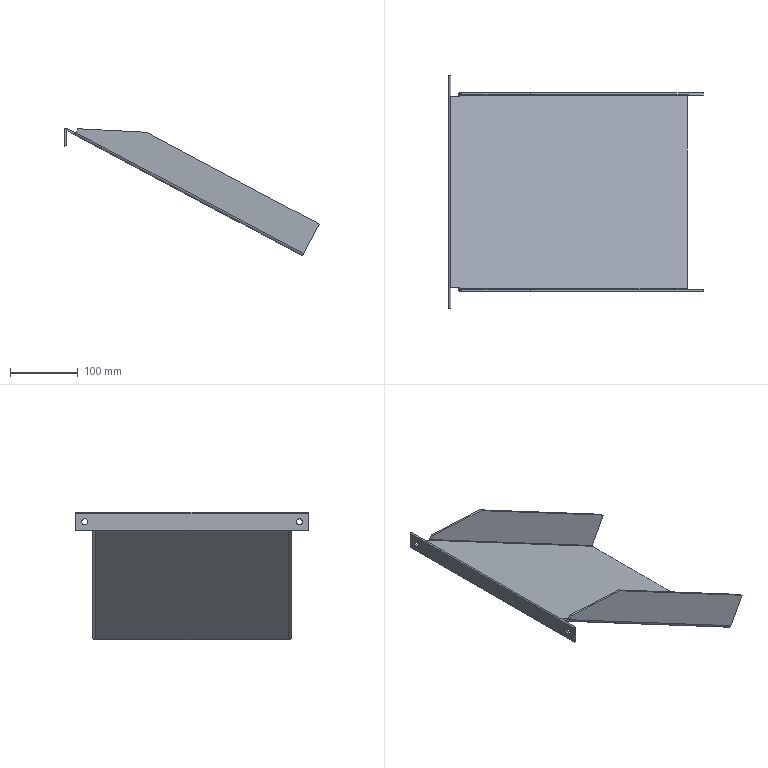Part | STEP file | lll_id3810_x_t | 1 solid | 27 faces | box 374.192 x 342 x 188.133 mm | volume 469805 mm3 | plane 20 | cylinder 7 | commonest cylinder face diameters 2 x2 8 x2 9 x2 3 x1
STEP:
#1=CARTESIAN_POINT('',(230.435,126.,-181.5));
#2=VERTEX_POINT('',#1);
#3=CARTESIAN_POINT('',(230.435,96.,-181.5));
#4=VERTEX_POINT('',#3);
#5=CARTESIAN_POINT('',(230.435,36.,-181.5));
#6=DIRECTION('',(0.,-1.,0.));
#7=VECTOR('',#6,1.);
#8=LINE('',#5,#7);
#9=EDGE_CURVE('',#2,#4,#8,.T.);
#10=ORIENTED_EDGE('',*,*,#9,.T.);
#11=CARTESIAN_POINT('',(230.435,96.,-183.996));
#12=VERTEX_POINT('',#11);
#13=CARTESIAN_POINT('',(230.435,96.,-193.833));
#14=DIRECTION('',(0.,0.,-1.));
#15=VECTOR('',#14,1.);
#16=LINE('',#13,#15);
#17=EDGE_CURVE('',#4,#12,#16,.T.);
#18=ORIENTED_EDGE('',*,*,#17,.T.);
#19=CARTESIAN_POINT('',(230.435,-186.,-183.996));
#20=VERTEX_POINT('',#19);
#21=CARTESIAN_POINT('',(230.435,-45.,-183.996));
#22=DIRECTION('',(0.,-1.,0.));
#23=VECTOR('',#22,1.);
#24=LINE('',#21,#23);
#25=EDGE_CURVE('',#12,#20,#24,.T.);
#26=ORIENTED_EDGE('',*,*,#25,.T.);
#27=CARTESIAN_POINT('',(230.435,-186.,-181.5));
#28=VERTEX_POINT('',#27);
#29=CARTESIAN_POINT('',(230.435,-186.,-193.833));
#30=DIRECTION('',(0.,0.,1.));
#31=VECTOR('',#30,1.);
#32=LINE('',#29,#31);
#33=EDGE_CURVE('',#20,#28,#32,.T.);
#34=ORIENTED_EDGE('',*,*,#33,.T.);
#35=CARTESIAN_POINT('',(230.435,-216.,-181.5));
#36=VERTEX_POINT('',#35);
#37=CARTESIAN_POINT('',(230.435,-201.,-181.5));
#38=DIRECTION('',(0.,-1.,0.));
#39=VECTOR('',#38,1.);
#40=LINE('',#37,#39);
#41=EDGE_CURVE('',#28,#36,#40,.T.);
#42=ORIENTED_EDGE('',*,*,#41,.T.);
#43=CARTESIAN_POINT('',(230.435,-216.,-206.128));
#44=VERTEX_POINT('',#43);
#45=CARTESIAN_POINT('',(230.435,-216.,-193.833));
#46=DIRECTION('',(0.,0.,1.));
#47=VECTOR('',#46,1.);
#48=LINE('',#45,#47);
#49=EDGE_CURVE('',#44,#36,#48,.T.);
#50=ORIENTED_EDGE('',*,*,#49,.F.);
#51=CARTESIAN_POINT('',(230.435,126.,-206.128));
#52=VERTEX_POINT('',#51);
#53=CARTESIAN_POINT('',(230.435,285.,-206.128));
#54=DIRECTION('',(0.,-1.,0.));
#55=VECTOR('',#54,1.);
#56=LINE('',#53,#55);
#57=EDGE_CURVE('',#52,#44,#56,.T.);
#58=ORIENTED_EDGE('',*,*,#57,.F.);
#59=CARTESIAN_POINT('',(230.435,126.,-193.833));
#60=DIRECTION('',(0.,0.,-1.));
#61=VECTOR('',#60,1.);
#62=LINE('',#59,#61);
#63=EDGE_CURVE('',#2,#52,#62,.T.);
#64=ORIENTED_EDGE('',*,*,#63,.F.);
#65=EDGE_LOOP('',(#10,#18,#26,#34,#42,#50,#58,#64));
#66=FACE_BOUND('',#65,.T.);
#67=CARTESIAN_POINT('',(230.435,113.,-189.565));
#68=VERTEX_POINT('',#67);
#69=CARTESIAN_POINT('',(230.435,113.,-194.083));
#70=DIRECTION('',(1.,0.,0.));
#71=DIRECTION('',(0.,0.,-1.));
#72=AXIS2_PLACEMENT_3D('',#69,#70,#71);
#73=ELLIPSE('',#72,4.517,4.5);
#74=EDGE_CURVE('',#68,#68,#73,.T.);
#75=ORIENTED_EDGE('',*,*,#74,.F.);
#76=EDGE_LOOP('',(#75));
#77=FACE_BOUND('',#76,.T.);
#78=CARTESIAN_POINT('',(230.435,-203.,-189.565));
#79=VERTEX_POINT('',#78);
#80=CARTESIAN_POINT('',(230.435,-203.,-194.083));
#81=DIRECTION('',(1.,0.,0.));
#82=DIRECTION('',(0.,0.,-1.));
#83=AXIS2_PLACEMENT_3D('',#80,#81,#82);
#84=ELLIPSE('',#83,4.517,4.5);
#85=EDGE_CURVE('',#79,#79,#84,.T.);
#86=ORIENTED_EDGE('',*,*,#85,.F.);
#87=EDGE_LOOP('',(#86));
#88=FACE_BOUND('',#87,.T.);
#89=CARTESIAN_POINT('',(230.435,-45.,-193.833));
#90=DIRECTION('',(1.,0.,0.));
#91=DIRECTION('',(0.,0.,-1.));
#92=AXIS2_PLACEMENT_3D('',#89,#90,#91);
#93=PLANE('',#92);
#94=ADVANCED_FACE('',(#66,#77,#88),#93,.T.);
#95=CARTESIAN_POINT('',(227.435,-216.,-206.391));
#96=VERTEX_POINT('',#95);
#97=CARTESIAN_POINT('',(227.435,-216.,-181.5));
#98=VERTEX_POINT('',#97);
#99=CARTESIAN_POINT('',(227.435,-216.,-173.216));
#100=DIRECTION('',(0.,0.,1.));
#101=VECTOR('',#100,1.);
#102=LINE('',#99,#101);
#103=EDGE_CURVE('',#96,#98,#102,.T.);
#104=ORIENTED_EDGE('',*,*,#103,.T.);
#105=CARTESIAN_POINT('',(227.435,126.,-181.5));
#106=VERTEX_POINT('',#105);
#107=CARTESIAN_POINT('',(227.435,-45.,-181.5));
#108=DIRECTION('',(0.,1.,0.));
#109=VECTOR('',#108,1.);
#110=LINE('',#107,#109);
#111=EDGE_CURVE('',#98,#106,#110,.T.);
#112=ORIENTED_EDGE('',*,*,#111,.T.);
#113=CARTESIAN_POINT('',(227.435,126.,-206.391));
#114=VERTEX_POINT('',#113);
#115=CARTESIAN_POINT('',(227.435,126.,-178.749));
#116=DIRECTION('',(0.,0.,-1.));
#117=VECTOR('',#116,1.);
#118=LINE('',#115,#117);
#119=EDGE_CURVE('',#106,#114,#118,.T.);
#120=ORIENTED_EDGE('',*,*,#119,.T.);
#121=CARTESIAN_POINT('',(227.435,110.,-206.391));
#122=DIRECTION('',(0.,-1.,0.));
#123=VECTOR('',#122,1.);
#124=LINE('',#121,#123);
#125=EDGE_CURVE('',#114,#96,#124,.T.);
#126=ORIENTED_EDGE('',*,*,#125,.T.);
#127=EDGE_LOOP('',(#104,#112,#120,#126));
#128=FACE_BOUND('',#127,.T.);
#129=CARTESIAN_POINT('',(227.435,113.,-198.862));
#130=VERTEX_POINT('',#129);
#131=CARTESIAN_POINT('',(227.435,113.,-194.345));
#132=DIRECTION('',(1.,0.,0.));
#133=DIRECTION('',(0.,0.,-1.));
#134=AXIS2_PLACEMENT_3D('',#131,#132,#133);
#135=ELLIPSE('',#134,4.517,4.5);
#136=EDGE_CURVE('',#130,#130,#135,.T.);
#137=ORIENTED_EDGE('',*,*,#136,.T.);
#138=EDGE_LOOP('',(#137));
#139=FACE_BOUND('',#138,.T.);
#140=CARTESIAN_POINT('',(227.435,-203.,-198.862));
#141=VERTEX_POINT('',#140);
#142=CARTESIAN_POINT('',(227.435,-203.,-194.345));
#143=DIRECTION('',(1.,0.,0.));
#144=DIRECTION('',(0.,0.,-1.));
#145=AXIS2_PLACEMENT_3D('',#142,#143,#144);
#146=ELLIPSE('',#145,4.517,4.5);
#147=EDGE_CURVE('',#141,#141,#146,.T.);
#148=ORIENTED_EDGE('',*,*,#147,.T.);
#149=EDGE_LOOP('',(#148));
#150=FACE_BOUND('',#149,.T.);
#151=CARTESIAN_POINT('',(227.435,110.,-170.446));
#152=DIRECTION('',(-1.,0.,0.));
#153=DIRECTION('',(0.,0.,-1.));
#154=AXIS2_PLACEMENT_3D('',#151,#152,#153);
#155=PLANE('',#154);
#156=ADVANCED_FACE('',(#128,#139,#150),#155,.T.);
#157=ORIENTED_EDGE('',*,*,#63,.T.);
#158=CARTESIAN_POINT('',(229.591,126.,-206.202));
#159=DIRECTION('',(-0.9962,0.,-0.08716));
#160=VECTOR('',#159,1.);
#161=LINE('',#158,#160);
#162=EDGE_CURVE('',#52,#114,#161,.T.);
#163=ORIENTED_EDGE('',*,*,#162,.T.);
#164=ORIENTED_EDGE('',*,*,#119,.F.);
#165=CARTESIAN_POINT('',(228.935,126.,-181.5));
#166=DIRECTION('',(0.,1.,0.));
#167=DIRECTION('',(-0.9962,0.,-0.08716));
#168=AXIS2_PLACEMENT_3D('',#165,#166,#167);
#169=CIRCLE('',#168,1.5);
#170=EDGE_CURVE('',#106,#2,#169,.T.);
#171=ORIENTED_EDGE('',*,*,#170,.T.);
#172=EDGE_LOOP('',(#157,#163,#164,#171));
#173=FACE_OUTER_BOUND('',#172,.T.);
#174=CARTESIAN_POINT('',(246.792,126.,-178.749));
#175=DIRECTION('',(0.,-1.,0.));
#176=DIRECTION('',(0.4226,0.,0.9063));
#177=AXIS2_PLACEMENT_3D('',#174,#175,#176);
#178=PLANE('',#177);
#179=ADVANCED_FACE('',(#173),#178,.F.);
#180=CARTESIAN_POINT('',(229.591,-216.,-206.202));
#181=DIRECTION('',(-0.9962,0.,-0.08716));
#182=VECTOR('',#181,1.);
#183=LINE('',#180,#182);
#184=EDGE_CURVE('',#44,#96,#183,.T.);
#185=ORIENTED_EDGE('',*,*,#184,.T.);
#186=ORIENTED_EDGE('',*,*,#125,.F.);
#187=ORIENTED_EDGE('',*,*,#162,.F.);
#188=ORIENTED_EDGE('',*,*,#57,.T.);
#189=EDGE_LOOP('',(#185,#186,#187,#188));
#190=FACE_OUTER_BOUND('',#189,.T.);
#191=CARTESIAN_POINT('',(229.591,285.,-206.202));
#192=DIRECTION('',(0.08716,0.,-0.9962));
#193=DIRECTION('',(0.,-1.,0.));
#194=AXIS2_PLACEMENT_3D('',#191,#192,#193);
#195=PLANE('',#194);
#196=ADVANCED_FACE('',(#190),#195,.T.);
#197=ORIENTED_EDGE('',*,*,#103,.F.);
#198=ORIENTED_EDGE('',*,*,#184,.F.);
#199=ORIENTED_EDGE('',*,*,#49,.T.);
#200=CARTESIAN_POINT('',(228.935,-216.,-181.5));
#201=DIRECTION('',(0.,-1.,0.));
#202=DIRECTION('',(-0.08716,0.,0.9962));
#203=AXIS2_PLACEMENT_3D('',#200,#201,#202);
#204=CIRCLE('',#203,1.5);
#205=EDGE_CURVE('',#36,#98,#204,.T.);
#206=ORIENTED_EDGE('',*,*,#205,.T.);
#207=EDGE_LOOP('',(#197,#198,#199,#206));
#208=FACE_OUTER_BOUND('',#207,.T.);
#209=CARTESIAN_POINT('',(226.705,-216.,-173.216));
#210=DIRECTION('',(0.,1.,0.));
#211=DIRECTION('',(0.08716,0.,-0.9962));
#212=AXIS2_PLACEMENT_3D('',#209,#210,#211);
#213=PLANE('',#212);
#214=ADVANCED_FACE('',(#208),#213,.F.);
#215=CARTESIAN_POINT('',(229.639,-186.,-180.176));
#216=VERTEX_POINT('',#215);
#217=CARTESIAN_POINT('',(242.945,-186.,-187.25));
#218=VERTEX_POINT('',#217);
#219=CARTESIAN_POINT('',(223.069,-186.,-176.682));
#220=DIRECTION('',(0.8829,0.,-0.4695));
#221=VECTOR('',#220,1.);
#222=LINE('',#219,#221);
#223=EDGE_CURVE('',#216,#218,#222,.T.);
#224=ORIENTED_EDGE('',*,*,#223,.T.);
#225=CARTESIAN_POINT('',(242.945,-187.,-187.25));
#226=VERTEX_POINT('',#225);
#227=CARTESIAN_POINT('',(242.945,92.,-187.25));
#228=DIRECTION('',(0.,-1.,0.));
#229=VECTOR('',#228,1.);
#230=LINE('',#227,#229);
#231=EDGE_CURVE('',#218,#226,#230,.T.);
#232=ORIENTED_EDGE('',*,*,#231,.T.);
#233=CARTESIAN_POINT('',(578.154,-187.,-365.484));
#234=VERTEX_POINT('',#233);
#235=CARTESIAN_POINT('',(228.807,-187.,-179.733));
#236=DIRECTION('',(0.8829,0.,-0.4695));
#237=VECTOR('',#236,1.);
#238=LINE('',#235,#237);
#239=EDGE_CURVE('',#226,#234,#238,.T.);
#240=ORIENTED_EDGE('',*,*,#239,.T.);
#241=CARTESIAN_POINT('',(578.154,97.,-365.484));
#242=VERTEX_POINT('',#241);
#243=CARTESIAN_POINT('',(578.154,-35.,-365.484));
#244=DIRECTION('',(0.,1.,0.));
#245=VECTOR('',#244,1.);
#246=LINE('',#243,#245);
#247=EDGE_CURVE('',#234,#242,#246,.T.);
#248=ORIENTED_EDGE('',*,*,#247,.T.);
#249=CARTESIAN_POINT('',(242.945,97.,-187.25));
#250=VERTEX_POINT('',#249);
#251=CARTESIAN_POINT('',(228.807,97.,-179.733));
#252=DIRECTION('',(-0.8829,0.,0.4695));
#253=VECTOR('',#252,1.);
#254=LINE('',#251,#253);
#255=EDGE_CURVE('',#242,#250,#254,.T.);
#256=ORIENTED_EDGE('',*,*,#255,.T.);
#257=CARTESIAN_POINT('',(242.945,96.,-187.25));
#258=VERTEX_POINT('',#257);
#259=CARTESIAN_POINT('',(242.945,-289.,-187.25));
#260=DIRECTION('',(0.,-1.,0.));
#261=VECTOR('',#260,1.);
#262=LINE('',#259,#261);
#263=EDGE_CURVE('',#250,#258,#262,.T.);
#264=ORIENTED_EDGE('',*,*,#263,.T.);
#265=CARTESIAN_POINT('',(229.639,96.,-180.176));
#266=VERTEX_POINT('',#265);
#267=CARTESIAN_POINT('',(228.631,96.,-179.64));
#268=DIRECTION('',(-0.8829,0.,0.4695));
#269=VECTOR('',#268,1.);
#270=LINE('',#267,#269);
#271=EDGE_CURVE('',#258,#266,#270,.T.);
#272=ORIENTED_EDGE('',*,*,#271,.T.);
#273=CARTESIAN_POINT('',(229.639,-45.,-180.176));
#274=DIRECTION('',(0.,-1.,0.));
#275=VECTOR('',#274,1.);
#276=LINE('',#273,#275);
#277=EDGE_CURVE('',#266,#216,#276,.T.);
#278=ORIENTED_EDGE('',*,*,#277,.T.);
#279=EDGE_LOOP('',(#224,#232,#240,#248,#256,#264,#272,#278));
#280=FACE_OUTER_BOUND('',#279,.T.);
#281=CARTESIAN_POINT('',(228.807,-35.,-179.733));
#282=DIRECTION('',(0.4695,0.,0.8829));
#283=DIRECTION('',(0.8829,0.,-0.4695));
#284=AXIS2_PLACEMENT_3D('',#281,#282,#283);
#285=PLANE('',#284);
#286=ADVANCED_FACE('',(#280),#285,.T.);
#287=ORIENTED_EDGE('',*,*,#271,.F.);
#288=CARTESIAN_POINT('',(241.537,96.,-189.899));
#289=VERTEX_POINT('',#288);
#290=CARTESIAN_POINT('',(242.945,96.,-187.25));
#291=DIRECTION('',(0.4695,0.,0.8829));
#292=VECTOR('',#291,1.);
#293=LINE('',#290,#292);
#294=EDGE_CURVE('',#289,#258,#293,.T.);
#295=ORIENTED_EDGE('',*,*,#294,.F.);
#296=CARTESIAN_POINT('',(227.399,96.,-182.382));
#297=DIRECTION('',(-0.8829,0.,0.4695));
#298=VECTOR('',#297,1.);
#299=LINE('',#296,#298);
#300=EDGE_CURVE('',#289,#12,#299,.T.);
#301=ORIENTED_EDGE('',*,*,#300,.T.);
#302=ORIENTED_EDGE('',*,*,#17,.F.);
#303=CARTESIAN_POINT('',(228.935,96.,-181.5));
#304=DIRECTION('',(0.,-1.,0.));
#305=DIRECTION('',(0.08716,0.,-0.9962));
#306=AXIS2_PLACEMENT_3D('',#303,#304,#305);
#307=CIRCLE('',#306,1.5);
#308=EDGE_CURVE('',#4,#266,#307,.T.);
#309=ORIENTED_EDGE('',*,*,#308,.T.);
#310=EDGE_LOOP('',(#287,#295,#301,#302,#309));
#311=FACE_OUTER_BOUND('',#310,.T.);
#312=CARTESIAN_POINT('',(228.563,96.,-179.768));
#313=DIRECTION('',(0.,-1.,0.));
#314=DIRECTION('',(0.9397,0.,-0.342));
#315=AXIS2_PLACEMENT_3D('',#312,#313,#314);
#316=PLANE('',#315);
#317=ADVANCED_FACE('',(#311),#316,.F.);
#318=CARTESIAN_POINT('',(228.935,-186.,-181.5));
#319=DIRECTION('',(0.,1.,0.));
#320=DIRECTION('',(0.9962,0.,0.08716));
#321=AXIS2_PLACEMENT_3D('',#318,#319,#320);
#322=CIRCLE('',#321,1.5);
#323=EDGE_CURVE('',#216,#28,#322,.T.);
#324=ORIENTED_EDGE('',*,*,#323,.T.);
#325=ORIENTED_EDGE('',*,*,#33,.F.);
#326=CARTESIAN_POINT('',(241.537,-186.,-189.899));
#327=VERTEX_POINT('',#326);
#328=CARTESIAN_POINT('',(227.399,-186.,-182.382));
#329=DIRECTION('',(0.8829,0.,-0.4695));
#330=VECTOR('',#329,1.);
#331=LINE('',#328,#330);
#332=EDGE_CURVE('',#20,#327,#331,.T.);
#333=ORIENTED_EDGE('',*,*,#332,.T.);
#334=CARTESIAN_POINT('',(242.945,-186.,-187.25));
#335=DIRECTION('',(0.4695,0.,0.8829));
#336=VECTOR('',#335,1.);
#337=LINE('',#334,#336);
#338=EDGE_CURVE('',#327,#218,#337,.T.);
#339=ORIENTED_EDGE('',*,*,#338,.T.);
#340=ORIENTED_EDGE('',*,*,#223,.F.);
#341=EDGE_LOOP('',(#324,#325,#333,#339,#340));
#342=FACE_OUTER_BOUND('',#341,.T.);
#343=CARTESIAN_POINT('',(232.324,-186.,-159.275));
#344=DIRECTION('',(0.,1.,0.));
#345=DIRECTION('',(-0.9848,0.,-0.1736));
#346=AXIS2_PLACEMENT_3D('',#343,#344,#345);
#347=PLANE('',#346);
#348=ADVANCED_FACE('',(#342),#347,.F.);
#349=ORIENTED_EDGE('',*,*,#111,.F.);
#350=ORIENTED_EDGE('',*,*,#205,.F.);
#351=ORIENTED_EDGE('',*,*,#41,.F.);
#352=ORIENTED_EDGE('',*,*,#323,.F.);
#353=ORIENTED_EDGE('',*,*,#277,.F.);
#354=ORIENTED_EDGE('',*,*,#308,.F.);
#355=ORIENTED_EDGE('',*,*,#9,.F.);
#356=ORIENTED_EDGE('',*,*,#170,.F.);
#357=EDGE_LOOP('',(#349,#350,#351,#352,#353,#354,#355,#356));
#358=FACE_OUTER_BOUND('',#357,.T.);
#359=CARTESIAN_POINT('',(228.935,36.,-181.5));
#360=DIRECTION('',(0.,-1.,0.));
#361=DIRECTION('',(0.9848,0.,0.1736));
#362=AXIS2_PLACEMENT_3D('',#359,#360,#361);
#363=CYLINDRICAL_SURFACE('',#362,1.5);
#364=ADVANCED_FACE('',(#358),#363,.T.);
#365=ORIENTED_EDGE('',*,*,#136,.F.);
#366=EDGE_LOOP('',(#365));
#367=FACE_BOUND('',#366,.T.);
#368=ORIENTED_EDGE('',*,*,#74,.T.);
#369=EDGE_LOOP('',(#368));
#370=FACE_BOUND('',#369,.T.);
#371=CARTESIAN_POINT('',(228.545,113.,-194.248));
#372=DIRECTION('',(-0.9962,0.,-0.08716));
#373=DIRECTION('',(0.,-1.,0.));
#374=AXIS2_PLACEMENT_3D('',#371,#372,#373);
#375=CYLINDRICAL_SURFACE('',#374,4.5);
#376=ADVANCED_FACE('',(#367,#370),#375,.F.);
#377=ORIENTED_EDGE('',*,*,#147,.F.);
#378=EDGE_LOOP('',(#377));
#379=FACE_BOUND('',#378,.T.);
#380=ORIENTED_EDGE('',*,*,#85,.T.);
#381=EDGE_LOOP('',(#380));
#382=FACE_BOUND('',#381,.T.);
#383=CARTESIAN_POINT('',(228.545,-203.,-194.248));
#384=DIRECTION('',(-0.9962,0.,-0.08716));
#385=DIRECTION('',(0.,-1.,0.));
#386=AXIS2_PLACEMENT_3D('',#383,#384,#385);
#387=CYLINDRICAL_SURFACE('',#386,4.5);
#388=ADVANCED_FACE('',(#379,#382),#387,.F.);
#389=CARTESIAN_POINT('',(347.494,-191.,-186.211));
#390=VERTEX_POINT('',#389);
#391=CARTESIAN_POINT('',(347.494,-188.,-186.211));
#392=VERTEX_POINT('',#391);
#393=CARTESIAN_POINT('',(347.494,-188.,-186.211));
#394=DIRECTION('',(0.,1.,0.));
#395=VECTOR('',#394,1.);
#396=LINE('',#393,#395);
#397=EDGE_CURVE('',#390,#392,#396,.T.);
#398=ORIENTED_EDGE('',*,*,#397,.F.);
#399=CARTESIAN_POINT('',(601.628,-191.,-321.337));
#400=VERTEX_POINT('',#399);
#401=CARTESIAN_POINT('',(404.484,-191.,-216.514));
#402=DIRECTION('',(0.8829,0.,-0.4695));
#403=VECTOR('',#402,1.);
#404=LINE('',#401,#403);
#405=EDGE_CURVE('',#390,#400,#404,.T.);
#406=ORIENTED_EDGE('',*,*,#405,.T.);
#407=CARTESIAN_POINT('',(601.628,-188.,-321.337));
#408=VERTEX_POINT('',#407);
#409=CARTESIAN_POINT('',(601.628,-35.,-321.337));
#410=DIRECTION('',(0.,-1.,0.));
#411=VECTOR('',#410,1.);
#412=LINE('',#409,#411);
#413=EDGE_CURVE('',#408,#400,#412,.T.);
#414=ORIENTED_EDGE('',*,*,#413,.F.);
#415=CARTESIAN_POINT('',(404.484,-188.,-216.514));
#416=DIRECTION('',(0.8829,0.,-0.4695));
#417=VECTOR('',#416,1.);
#418=LINE('',#415,#417);
#419=EDGE_CURVE('',#392,#408,#418,.T.);
#420=ORIENTED_EDGE('',*,*,#419,.F.);
#421=EDGE_LOOP('',(#398,#406,#414,#420));
#422=FACE_OUTER_BOUND('',#421,.T.);
#423=CARTESIAN_POINT('',(404.484,-188.,-216.514));
#424=DIRECTION('',(-0.4695,0.,-0.8829));
#425=DIRECTION('',(0.8829,0.,-0.4695));
#426=AXIS2_PLACEMENT_3D('',#423,#424,#425);
#427=PLANE('',#426);
#428=ADVANCED_FACE('',(#422),#427,.F.);
#429=CARTESIAN_POINT('',(246.317,-188.,-180.909));
#430=VERTEX_POINT('',#429);
#431=CARTESIAN_POINT('',(246.317,-191.,-180.909));
#432=VERTEX_POINT('',#431);
#433=CARTESIAN_POINT('',(246.317,-148.,-180.909));
#434=DIRECTION('',(0.,-1.,0.));
#435=VECTOR('',#434,1.);
#436=LINE('',#433,#435);
#437=EDGE_CURVE('',#430,#432,#436,.T.);
#438=ORIENTED_EDGE('',*,*,#437,.F.);
#439=CARTESIAN_POINT('',(243.415,-188.,-186.368));
#440=VERTEX_POINT('',#439);
#441=CARTESIAN_POINT('',(242.476,-188.,-188.133));
#442=DIRECTION('',(0.4695,0.,0.8829));
#443=VECTOR('',#442,1.);
#444=LINE('',#441,#443);
#445=EDGE_CURVE('',#440,#430,#444,.T.);
#446=ORIENTED_EDGE('',*,*,#445,.F.);
#447=CARTESIAN_POINT('',(243.415,-187.,-186.368));
#448=DIRECTION('',(-0.8829,0.,0.4695));
#449=DIRECTION('',(0.4695,0.,0.8829));
#450=AXIS2_PLACEMENT_3D('',#447,#448,#449);
#451=CIRCLE('',#450,1.);
#452=EDGE_CURVE('',#226,#440,#451,.T.);
#453=ORIENTED_EDGE('',*,*,#452,.F.);
#454=ORIENTED_EDGE('',*,*,#231,.F.);
#455=ORIENTED_EDGE('',*,*,#338,.F.);
#456=CARTESIAN_POINT('',(241.537,-187.,-189.899));
#457=VERTEX_POINT('',#456);
#458=CARTESIAN_POINT('',(241.537,55.,-189.899));
#459=DIRECTION('',(0.,-1.,0.));
#460=VECTOR('',#459,1.);
#461=LINE('',#458,#460);
#462=EDGE_CURVE('',#327,#457,#461,.T.);
#463=ORIENTED_EDGE('',*,*,#462,.T.);
#464=CARTESIAN_POINT('',(243.415,-191.,-186.368));
#465=VERTEX_POINT('',#464);
#466=CARTESIAN_POINT('',(243.415,-187.,-186.368));
#467=DIRECTION('',(-0.8829,0.,0.4695));
#468=DIRECTION('',(0.4695,0.,0.8829));
#469=AXIS2_PLACEMENT_3D('',#466,#467,#468);
#470=CIRCLE('',#469,4.);
#471=EDGE_CURVE('',#457,#465,#470,.T.);
#472=ORIENTED_EDGE('',*,*,#471,.T.);
#473=CARTESIAN_POINT('',(242.945,-191.,-187.25));
#474=DIRECTION('',(0.4695,0.,0.8829));
#475=VECTOR('',#474,1.);
#476=LINE('',#473,#475);
#477=EDGE_CURVE('',#465,#432,#476,.T.);
#478=ORIENTED_EDGE('',*,*,#477,.T.);
#479=EDGE_LOOP('',(#438,#446,#453,#454,#455,#463,#472,#478));
#480=FACE_OUTER_BOUND('',#479,.T.);
#481=CARTESIAN_POINT('',(242.945,-148.,-187.25));
#482=DIRECTION('',(-0.8829,0.,0.4695));
#483=DIRECTION('',(0.,-1.,0.));
#484=AXIS2_PLACEMENT_3D('',#481,#482,#483);
#485=PLANE('',#484);
#486=ADVANCED_FACE('',(#480),#485,.T.);
#487=CARTESIAN_POINT('',(246.317,98.,-180.909));
#488=VERTEX_POINT('',#487);
#489=CARTESIAN_POINT('',(246.317,101.,-180.909));
#490=VERTEX_POINT('',#489);
#491=CARTESIAN_POINT('',(246.317,98.,-180.909));
#492=DIRECTION('',(0.,1.,0.));
#493=VECTOR('',#492,1.);
#494=LINE('',#491,#493);
#495=EDGE_CURVE('',#488,#490,#494,.T.);
#496=ORIENTED_EDGE('',*,*,#495,.T.);
#497=CARTESIAN_POINT('',(243.415,101.,-186.368));
#498=VERTEX_POINT('',#497);
#499=CARTESIAN_POINT('',(243.415,101.,-186.368));
#500=DIRECTION('',(-0.4695,0.,-0.8829));
#501=VECTOR('',#500,1.);
#502=LINE('',#499,#501);
#503=EDGE_CURVE('',#490,#498,#502,.T.);
#504=ORIENTED_EDGE('',*,*,#503,.T.);
#505=CARTESIAN_POINT('',(241.537,97.,-189.899));
#506=VERTEX_POINT('',#505);
#507=CARTESIAN_POINT('',(243.415,97.,-186.368));
#508=DIRECTION('',(-0.8829,0.,0.4695));
#509=DIRECTION('',(0.4695,0.,0.8829));
#510=AXIS2_PLACEMENT_3D('',#507,#508,#509);
#511=CIRCLE('',#510,4.);
#512=EDGE_CURVE('',#498,#506,#511,.T.);
#513=ORIENTED_EDGE('',*,*,#512,.T.);
#514=CARTESIAN_POINT('',(241.537,-215.,-189.899));
#515=DIRECTION('',(0.,-1.,0.));
#516=VECTOR('',#515,1.);
#517=LINE('',#514,#516);
#518=EDGE_CURVE('',#506,#289,#517,.T.);
#519=ORIENTED_EDGE('',*,*,#518,.T.);
#520=ORIENTED_EDGE('',*,*,#294,.T.);
#521=ORIENTED_EDGE('',*,*,#263,.F.);
#522=CARTESIAN_POINT('',(243.415,98.,-186.368));
#523=VERTEX_POINT('',#522);
#524=CARTESIAN_POINT('',(243.415,97.,-186.368));
#525=DIRECTION('',(-0.8829,0.,0.4695));
#526=DIRECTION('',(0.4695,0.,0.8829));
#527=AXIS2_PLACEMENT_3D('',#524,#525,#526);
#528=CIRCLE('',#527,1.);
#529=EDGE_CURVE('',#523,#250,#528,.T.);
#530=ORIENTED_EDGE('',*,*,#529,.F.);
#531=CARTESIAN_POINT('',(243.415,98.,-186.368));
#532=DIRECTION('',(-0.4695,0.,-0.8829));
#533=VECTOR('',#532,1.);
#534=LINE('',#531,#533);
#535=EDGE_CURVE('',#488,#523,#534,.T.);
#536=ORIENTED_EDGE('',*,*,#535,.F.);
#537=EDGE_LOOP('',(#496,#504,#513,#519,#520,#521,#530,#536));
#538=FACE_OUTER_BOUND('',#537,.T.);
#539=CARTESIAN_POINT('',(243.415,98.,-186.368));
#540=DIRECTION('',(-0.8829,0.,0.4695));
#541=DIRECTION('',(0.4695,0.,0.8829));
#542=AXIS2_PLACEMENT_3D('',#539,#540,#541);
#543=PLANE('',#542);
#544=ADVANCED_FACE('',(#538),#543,.T.);
#545=CARTESIAN_POINT('',(347.494,98.,-186.211));
#546=VERTEX_POINT('',#545);
#547=CARTESIAN_POINT('',(347.494,101.,-186.211));
#548=VERTEX_POINT('',#547);
#549=CARTESIAN_POINT('',(347.494,98.,-186.211));
#550=DIRECTION('',(0.,1.,0.));
#551=VECTOR('',#550,1.);
#552=LINE('',#549,#551);
#553=EDGE_CURVE('',#546,#548,#552,.T.);
#554=ORIENTED_EDGE('',*,*,#553,.F.);
#555=CARTESIAN_POINT('',(601.628,98.,-321.337));
#556=VERTEX_POINT('',#555);
#557=CARTESIAN_POINT('',(404.484,98.,-216.514));
#558=DIRECTION('',(-0.8829,0.,0.4695));
#559=VECTOR('',#558,1.);
#560=LINE('',#557,#559);
#561=EDGE_CURVE('',#556,#546,#560,.T.);
#562=ORIENTED_EDGE('',*,*,#561,.F.);
#563=CARTESIAN_POINT('',(601.628,101.,-321.337));
#564=VERTEX_POINT('',#563);
#565=CARTESIAN_POINT('',(601.628,98.,-321.337));
#566=DIRECTION('',(0.,1.,0.));
#567=VECTOR('',#566,1.);
#568=LINE('',#565,#567);
#569=EDGE_CURVE('',#556,#564,#568,.T.);
#570=ORIENTED_EDGE('',*,*,#569,.T.);
#571=CARTESIAN_POINT('',(404.484,101.,-216.514));
#572=DIRECTION('',(-0.8829,0.,0.4695));
#573=VECTOR('',#572,1.);
#574=LINE('',#571,#573);
#575=EDGE_CURVE('',#564,#548,#574,.T.);
#576=ORIENTED_EDGE('',*,*,#575,.T.);
#577=EDGE_LOOP('',(#554,#562,#570,#576));
#578=FACE_OUTER_BOUND('',#577,.T.);
#579=CARTESIAN_POINT('',(404.484,98.,-216.514));
#580=DIRECTION('',(-0.4695,0.,-0.8829));
#581=DIRECTION('',(-0.8829,0.,0.4695));
#582=AXIS2_PLACEMENT_3D('',#579,#580,#581);
#583=PLANE('',#582);
#584=ADVANCED_FACE('',(#578),#583,.F.);
#585=CARTESIAN_POINT('',(147.708,-188.,-175.741));
#586=DIRECTION('',(-0.9986,0.,0.05234));
#587=VECTOR('',#586,1.);
#588=LINE('',#585,#587);
#589=EDGE_CURVE('',#392,#430,#588,.T.);
#590=ORIENTED_EDGE('',*,*,#589,.F.);
#591=ORIENTED_EDGE('',*,*,#419,.T.);
#592=CARTESIAN_POINT('',(578.623,-188.,-364.601));
#593=VERTEX_POINT('',#592);
#594=CARTESIAN_POINT('',(577.684,-188.,-366.367));
#595=DIRECTION('',(-0.4695,0.,-0.8829));
#596=VECTOR('',#595,1.);
#597=LINE('',#594,#596);
#598=EDGE_CURVE('',#408,#593,#597,.T.);
#599=ORIENTED_EDGE('',*,*,#598,.T.);
#600=CARTESIAN_POINT('',(150.584,-188.,-137.009));
#601=DIRECTION('',(-0.8829,0.,0.4695));
#602=VECTOR('',#601,1.);
#603=LINE('',#600,#602);
#604=EDGE_CURVE('',#593,#440,#603,.T.);
#605=ORIENTED_EDGE('',*,*,#604,.T.);
#606=ORIENTED_EDGE('',*,*,#445,.T.);
#607=EDGE_LOOP('',(#590,#591,#599,#605,#606));
#608=FACE_OUTER_BOUND('',#607,.T.);
#609=CARTESIAN_POINT('',(149.645,-188.,-138.775));
#610=DIRECTION('',(0.,-1.,0.));
#611=DIRECTION('',(0.2924,0.,-0.9563));
#612=AXIS2_PLACEMENT_3D('',#609,#610,#611);
#613=PLANE('',#612);
#614=ADVANCED_FACE('',(#608),#613,.F.);
#615=CARTESIAN_POINT('',(147.983,98.,-175.755));
#616=DIRECTION('',(-0.9986,0.,0.05234));
#617=VECTOR('',#616,1.);
#618=LINE('',#615,#617);
#619=EDGE_CURVE('',#546,#488,#618,.T.);
#620=ORIENTED_EDGE('',*,*,#619,.T.);
#621=ORIENTED_EDGE('',*,*,#535,.T.);
#622=CARTESIAN_POINT('',(578.623,98.,-364.601));
#623=VERTEX_POINT('',#622);
#624=CARTESIAN_POINT('',(150.767,98.,-137.106));
#625=DIRECTION('',(0.8829,0.,-0.4695));
#626=VECTOR('',#625,1.);
#627=LINE('',#624,#626);
#628=EDGE_CURVE('',#523,#623,#627,.T.);
#629=ORIENTED_EDGE('',*,*,#628,.T.);
#630=CARTESIAN_POINT('',(577.782,98.,-366.184));
#631=DIRECTION('',(0.4695,0.,0.8829));
#632=VECTOR('',#631,1.);
#633=LINE('',#630,#632);
#634=EDGE_CURVE('',#623,#556,#633,.T.);
#635=ORIENTED_EDGE('',*,*,#634,.T.);
#636=ORIENTED_EDGE('',*,*,#561,.T.);
#637=EDGE_LOOP('',(#620,#621,#629,#635,#636));
#638=FACE_OUTER_BOUND('',#637,.T.);
#639=CARTESIAN_POINT('',(149.925,98.,-138.689));
#640=DIRECTION('',(0.,1.,0.));
#641=DIRECTION('',(-0.2924,0.,0.9563));
#642=AXIS2_PLACEMENT_3D('',#639,#640,#641);
#643=PLANE('',#642);
#644=ADVANCED_FACE('',(#638),#643,.F.);
#645=ORIENTED_EDGE('',*,*,#405,.F.);
#646=CARTESIAN_POINT('',(147.708,-191.,-175.741));
#647=DIRECTION('',(0.9986,0.,-0.05234));
#648=VECTOR('',#647,1.);
#649=LINE('',#646,#648);
#650=EDGE_CURVE('',#432,#390,#649,.T.);
#651=ORIENTED_EDGE('',*,*,#650,.F.);
#652=ORIENTED_EDGE('',*,*,#477,.F.);
#653=CARTESIAN_POINT('',(578.623,-191.,-364.601));
#654=VERTEX_POINT('',#653);
#655=CARTESIAN_POINT('',(149.812,-191.,-136.598));
#656=DIRECTION('',(-0.8829,0.,0.4695));
#657=VECTOR('',#656,1.);
#658=LINE('',#655,#657);
#659=EDGE_CURVE('',#654,#465,#658,.T.);
#660=ORIENTED_EDGE('',*,*,#659,.F.);
#661=CARTESIAN_POINT('',(577.684,-191.,-366.367));
#662=DIRECTION('',(-0.4695,0.,-0.8829));
#663=VECTOR('',#662,1.);
#664=LINE('',#661,#663);
#665=EDGE_CURVE('',#400,#654,#664,.T.);
#666=ORIENTED_EDGE('',*,*,#665,.F.);
#667=EDGE_LOOP('',(#645,#651,#652,#660,#666));
#668=FACE_OUTER_BOUND('',#667,.T.);
#669=CARTESIAN_POINT('',(149.645,-191.,-138.775));
#670=DIRECTION('',(0.,-1.,0.));
#671=DIRECTION('',(0.2924,0.,-0.9563));
#672=AXIS2_PLACEMENT_3D('',#669,#670,#671);
#673=PLANE('',#672);
#674=ADVANCED_FACE('',(#668),#673,.T.);
#675=ORIENTED_EDGE('',*,*,#503,.F.);
#676=CARTESIAN_POINT('',(147.983,101.,-175.755));
#677=DIRECTION('',(0.9986,0.,-0.05234));
#678=VECTOR('',#677,1.);
#679=LINE('',#676,#678);
#680=EDGE_CURVE('',#490,#548,#679,.T.);
#681=ORIENTED_EDGE('',*,*,#680,.T.);
#682=ORIENTED_EDGE('',*,*,#575,.F.);
#683=CARTESIAN_POINT('',(578.623,101.,-364.601));
#684=VERTEX_POINT('',#683);
#685=CARTESIAN_POINT('',(577.782,101.,-366.184));
#686=DIRECTION('',(0.4695,0.,0.8829));
#687=VECTOR('',#686,1.);
#688=LINE('',#685,#687);
#689=EDGE_CURVE('',#684,#564,#688,.T.);
#690=ORIENTED_EDGE('',*,*,#689,.F.);
#691=CARTESIAN_POINT('',(149.812,101.,-136.598));
#692=DIRECTION('',(0.8829,0.,-0.4695));
#693=VECTOR('',#692,1.);
#694=LINE('',#691,#693);
#695=EDGE_CURVE('',#498,#684,#694,.T.);
#696=ORIENTED_EDGE('',*,*,#695,.F.);
#697=EDGE_LOOP('',(#675,#681,#682,#690,#696));
#698=FACE_OUTER_BOUND('',#697,.T.);
#699=CARTESIAN_POINT('',(149.925,101.,-138.689));
#700=DIRECTION('',(0.,1.,0.));
#701=DIRECTION('',(-0.2924,0.,0.9563));
#702=AXIS2_PLACEMENT_3D('',#699,#700,#701);
#703=PLANE('',#702);
#704=ADVANCED_FACE('',(#698),#703,.T.);
#705=ORIENTED_EDGE('',*,*,#25,.F.);
#706=ORIENTED_EDGE('',*,*,#300,.F.);
#707=ORIENTED_EDGE('',*,*,#518,.F.);
#708=CARTESIAN_POINT('',(576.746,97.,-368.133));
#709=VERTEX_POINT('',#708);
#710=CARTESIAN_POINT('',(227.399,97.,-182.382));
#711=DIRECTION('',(-0.8829,0.,0.4695));
#712=VECTOR('',#711,1.);
#713=LINE('',#710,#712);
#714=EDGE_CURVE('',#709,#506,#713,.T.);
#715=ORIENTED_EDGE('',*,*,#714,.F.);
#716=CARTESIAN_POINT('',(576.746,-187.,-368.133));
#717=VERTEX_POINT('',#716);
#718=CARTESIAN_POINT('',(576.746,-35.,-368.133));
#719=DIRECTION('',(0.,1.,0.));
#720=VECTOR('',#719,1.);
#721=LINE('',#718,#720);
#722=EDGE_CURVE('',#717,#709,#721,.T.);
#723=ORIENTED_EDGE('',*,*,#722,.F.);
#724=CARTESIAN_POINT('',(227.399,-187.,-182.382));
#725=DIRECTION('',(0.8829,0.,-0.4695));
#726=VECTOR('',#725,1.);
#727=LINE('',#724,#726);
#728=EDGE_CURVE('',#457,#717,#727,.T.);
#729=ORIENTED_EDGE('',*,*,#728,.F.);
#730=ORIENTED_EDGE('',*,*,#462,.F.);
#731=ORIENTED_EDGE('',*,*,#332,.F.);
#732=EDGE_LOOP('',(#705,#706,#707,#715,#723,#729,#730,#731));
#733=FACE_OUTER_BOUND('',#732,.T.);
#734=CARTESIAN_POINT('',(227.399,-35.,-182.382));
#735=DIRECTION('',(0.4695,0.,0.8829));
#736=DIRECTION('',(0.8829,0.,-0.4695));
#737=AXIS2_PLACEMENT_3D('',#734,#735,#736);
#738=PLANE('',#737);
#739=ADVANCED_FACE('',(#733),#738,.F.);
#740=ORIENTED_EDGE('',*,*,#722,.T.);
#741=CARTESIAN_POINT('',(578.623,97.,-364.601));
#742=DIRECTION('',(0.8829,0.,-0.4695));
#743=DIRECTION('',(0.4695,0.,0.8829));
#744=AXIS2_PLACEMENT_3D('',#741,#742,#743);
#745=CIRCLE('',#744,4.);
#746=EDGE_CURVE('',#709,#684,#745,.T.);
#747=ORIENTED_EDGE('',*,*,#746,.T.);
#748=ORIENTED_EDGE('',*,*,#689,.T.);
#749=ORIENTED_EDGE('',*,*,#569,.F.);
#750=ORIENTED_EDGE('',*,*,#634,.F.);
#751=CARTESIAN_POINT('',(578.623,97.,-364.601));
#752=DIRECTION('',(0.8829,0.,-0.4695));
#753=DIRECTION('',(0.4695,0.,0.8829));
#754=AXIS2_PLACEMENT_3D('',#751,#752,#753);
#755=CIRCLE('',#754,1.);
#756=EDGE_CURVE('',#242,#623,#755,.T.);
#757=ORIENTED_EDGE('',*,*,#756,.F.);
#758=ORIENTED_EDGE('',*,*,#247,.F.);
#759=CARTESIAN_POINT('',(578.623,-187.,-364.601));
#760=DIRECTION('',(0.8829,0.,-0.4695));
#761=DIRECTION('',(0.4695,0.,0.8829));
#762=AXIS2_PLACEMENT_3D('',#759,#760,#761);
#763=CIRCLE('',#762,1.);
#764=EDGE_CURVE('',#593,#234,#763,.T.);
#765=ORIENTED_EDGE('',*,*,#764,.F.);
#766=ORIENTED_EDGE('',*,*,#598,.F.);
#767=ORIENTED_EDGE('',*,*,#413,.T.);
#768=ORIENTED_EDGE('',*,*,#665,.T.);
#769=CARTESIAN_POINT('',(578.623,-187.,-364.601));
#770=DIRECTION('',(0.8829,0.,-0.4695));
#771=DIRECTION('',(0.4695,0.,0.8829));
#772=AXIS2_PLACEMENT_3D('',#769,#770,#771);
#773=CIRCLE('',#772,4.);
#774=EDGE_CURVE('',#654,#717,#773,.T.);
#775=ORIENTED_EDGE('',*,*,#774,.T.);
#776=EDGE_LOOP('',(#740,#747,#748,#749,#750,#757,#758,#765,#766,#767,#768,#775));
#777=FACE_OUTER_BOUND('',#776,.T.);
#778=CARTESIAN_POINT('',(578.154,-35.,-365.484));
#779=DIRECTION('',(-0.8829,0.,0.4695));
#780=DIRECTION('',(0.,-1.,0.));
#781=AXIS2_PLACEMENT_3D('',#778,#779,#780);
#782=PLANE('',#781);
#783=ADVANCED_FACE('',(#777),#782,.F.);
#784=ORIENTED_EDGE('',*,*,#628,.F.);
#785=ORIENTED_EDGE('',*,*,#529,.T.);
#786=ORIENTED_EDGE('',*,*,#255,.F.);
#787=ORIENTED_EDGE('',*,*,#756,.T.);
#788=EDGE_LOOP('',(#784,#785,#786,#787));
#789=FACE_OUTER_BOUND('',#788,.T.);
#790=CARTESIAN_POINT('',(149.812,97.,-136.598));
#791=DIRECTION('',(-0.8829,0.,0.4695));
#792=DIRECTION('',(0.4695,0.,0.8829));
#793=AXIS2_PLACEMENT_3D('',#790,#791,#792);
#794=CYLINDRICAL_SURFACE('',#793,1.);
#795=ADVANCED_FACE('',(#789),#794,.F.);
#796=ORIENTED_EDGE('',*,*,#239,.F.);
#797=ORIENTED_EDGE('',*,*,#452,.T.);
#798=ORIENTED_EDGE('',*,*,#604,.F.);
#799=ORIENTED_EDGE('',*,*,#764,.T.);
#800=EDGE_LOOP('',(#796,#797,#798,#799));
#801=FACE_OUTER_BOUND('',#800,.T.);
#802=CARTESIAN_POINT('',(149.812,-187.,-136.598));
#803=DIRECTION('',(0.8829,0.,-0.4695));
#804=DIRECTION('',(-0.4695,0.,-0.8829));
#805=AXIS2_PLACEMENT_3D('',#802,#803,#804);
#806=CYLINDRICAL_SURFACE('',#805,1.);
#807=ADVANCED_FACE('',(#801),#806,.F.);
#808=ORIENTED_EDGE('',*,*,#695,.T.);
#809=ORIENTED_EDGE('',*,*,#746,.F.);
#810=ORIENTED_EDGE('',*,*,#714,.T.);
#811=ORIENTED_EDGE('',*,*,#512,.F.);
#812=EDGE_LOOP('',(#808,#809,#810,#811));
#813=FACE_OUTER_BOUND('',#812,.T.);
#814=CARTESIAN_POINT('',(149.812,97.,-136.598));
#815=DIRECTION('',(-0.8829,0.,0.4695));
#816=DIRECTION('',(0.4695,0.,0.8829));
#817=AXIS2_PLACEMENT_3D('',#814,#815,#816);
#818=CYLINDRICAL_SURFACE('',#817,4.);
#819=ADVANCED_FACE('',(#813),#818,.T.);
#820=ORIENTED_EDGE('',*,*,#728,.T.);
#821=ORIENTED_EDGE('',*,*,#774,.F.);
#822=ORIENTED_EDGE('',*,*,#659,.T.);
#823=ORIENTED_EDGE('',*,*,#471,.F.);
#824=EDGE_LOOP('',(#820,#821,#822,#823));
#825=FACE_OUTER_BOUND('',#824,.T.);
#826=CARTESIAN_POINT('',(149.812,-187.,-136.598));
#827=DIRECTION('',(0.8829,0.,-0.4695));
#828=DIRECTION('',(-0.4695,0.,-0.8829));
#829=AXIS2_PLACEMENT_3D('',#826,#827,#828);
#830=CYLINDRICAL_SURFACE('',#829,4.);
#831=ADVANCED_FACE('',(#825),#830,.T.);
#832=ORIENTED_EDGE('',*,*,#495,.F.);
#833=ORIENTED_EDGE('',*,*,#619,.F.);
#834=ORIENTED_EDGE('',*,*,#553,.T.);
#835=ORIENTED_EDGE('',*,*,#680,.F.);
#836=EDGE_LOOP('',(#832,#833,#834,#835));
#837=FACE_OUTER_BOUND('',#836,.T.);
#838=CARTESIAN_POINT('',(197.557,0.,-178.353));
#839=DIRECTION('',(0.05234,0.,0.9986));
#840=DIRECTION('',(0.9986,0.,-0.05234));
#841=AXIS2_PLACEMENT_3D('',#838,#839,#840);
#842=PLANE('',#841);
#843=ADVANCED_FACE('',(#837),#842,.T.);
#844=ORIENTED_EDGE('',*,*,#397,.T.);
#845=ORIENTED_EDGE('',*,*,#589,.T.);
#846=ORIENTED_EDGE('',*,*,#437,.T.);
#847=ORIENTED_EDGE('',*,*,#650,.T.);
#848=EDGE_LOOP('',(#844,#845,#846,#847));
#849=FACE_OUTER_BOUND('',#848,.T.);
#850=CARTESIAN_POINT('',(197.557,0.,-178.353));
#851=DIRECTION('',(0.05234,0.,0.9986));
#852=DIRECTION('',(0.9986,0.,-0.05234));
#853=AXIS2_PLACEMENT_3D('',#850,#851,#852);
#854=PLANE('',#853);
#855=ADVANCED_FACE('',(#849),#854,.T.);
#856=CLOSED_SHELL('',(#94,#156,#179,#196,#214,#286,#317,#348,#364,#376,#388,#428,#486,#544,#584,#614,#644,#674,#704,#739,#783,#795,#807,#819,#831,#843,#855));
#857=MANIFOLD_SOLID_BREP('',#856);
#858=(LENGTH_UNIT()NAMED_UNIT(*)SI_UNIT(.MILLI.,.METRE.));
#859=UNCERTAINTY_MEASURE_WITH_UNIT(LENGTH_MEASURE(0.00002561),#858,'','');
#860=(NAMED_UNIT(*)PLANE_ANGLE_UNIT()SI_UNIT($,.RADIAN.));
#861=PLANE_ANGLE_MEASURE_WITH_UNIT(PLANE_ANGLE_MEASURE(0.01745),#860);
#862=DIMENSIONAL_EXPONENTS(0.,0.,0.,0.,0.,0.,0.);
#863=(CONVERSION_BASED_UNIT('DEGREE',#861)NAMED_UNIT(#862)PLANE_ANGLE_UNIT());
#864=(NAMED_UNIT(*)SI_UNIT($,.STERADIAN.)SOLID_ANGLE_UNIT());
#865=(GEOMETRIC_REPRESENTATION_CONTEXT(3)GLOBAL_UNCERTAINTY_ASSIGNED_CONTEXT((#859))GLOBAL_UNIT_ASSIGNED_CONTEXT((#858,#863,#864))REPRESENTATION_CONTEXT('',''));
#866=ADVANCED_BREP_SHAPE_REPRESENTATION('',(#857),#865);